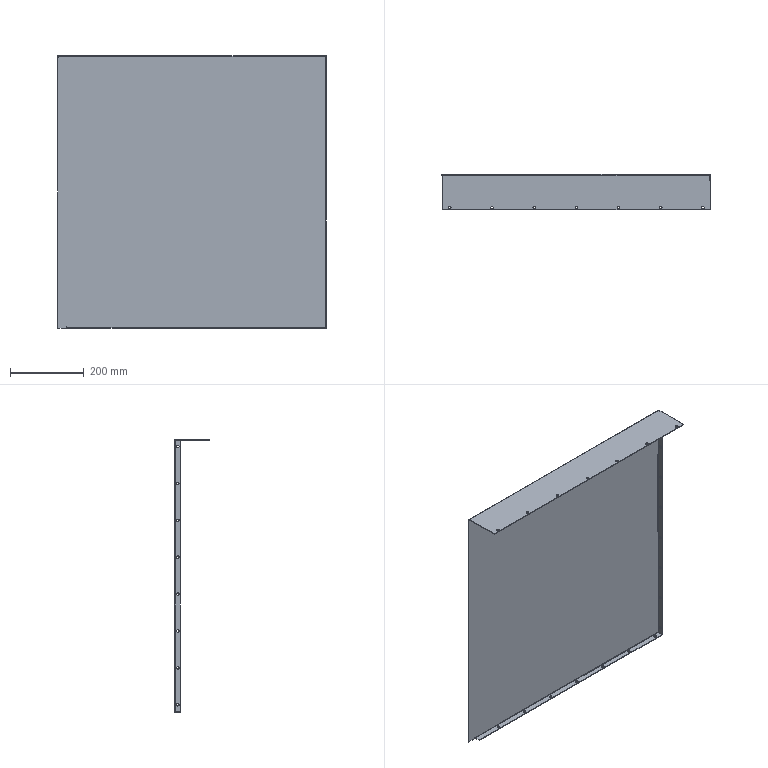Part | STEP file | Top Cover 3 | 1 solid | 77 faces | box 728 x 97 x 738 mm | volume 1251055 mm3 | cylinder 53 | plane 24 | commonest cylinder face diameters 7 x44 1 x6 5 x3